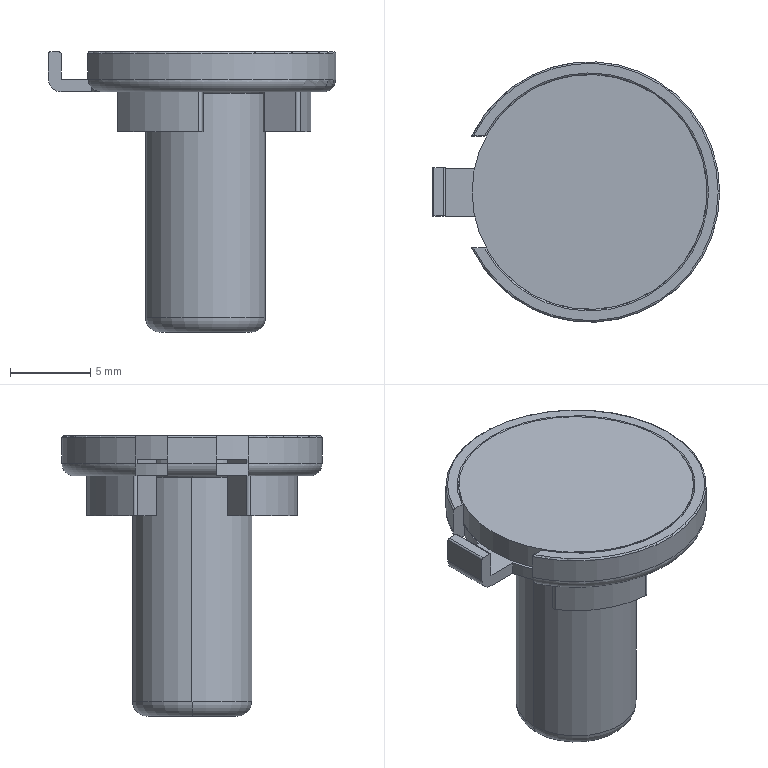NC program | NX | posted with a generic post | part box 17.958 x 16.273 x 17.5 mm
Lines 8183 to 8588 of 11029:
(刀补1 , TOOL : D4)
N16346 T04 M6
N16348 G54
N16350 G17 G0 G90 X3.736 Y7.769 S6500 M3
N16352 G43 Z30. H4
N16354 Z1.
N16356 G94 G1 X3.87 Y7.711 Z0.992 F1000.
N16358 X4.743 Y7.207 Z0.94
N16360 X5.551 Y6.604 Z0.887
N16362 X6.284 Y5.911 Z0.834
N16364 X6.931 Y5.138 Z0.781
N16366 X7.162 Y4.793 Z0.759
N16368 X7.279 Y4.617 Z0.748
N16370 X7.472 Y4.131 Z0.721
N16372 X7.546 Y3.613 Z0.693
N16374 X7.497 Y3.092 Z0.666
N16376 X7.328 Y2.597 Z0.638
N16378 X7.048 Y2.155 Z0.611
N16380 X6.673 Y1.791 Z0.584
N16382 X4.919 Y0.695 Z0.475
N16384 X4.963 Y0.382 Z0.459
N16386 Y-0.382 Z0.419
N16388 X4.919 Y-0.695 Z0.402
N16390 X6.673 Y-1.791 Z0.294
N16392 X7.048 Y-2.155 Z0.266
N16394 X7.328 Y-2.597 Z0.239
N16396 X7.497 Y-3.092 Z0.211
N16398 X7.546 Y-3.613 Z0.184
N16400 X7.472 Y-4.131 Z0.157
N16402 X7.279 Y-4.617 Z0.129
N16404 X7.162 Y-4.793 Z0.118
N16406 X6.931 Y-5.138 Z0.096
N16408 X6.284 Y-5.911 Z0.044
N16410 X5.551 Y-6.604 Z-0.009
N16412 X4.743 Y-7.207 Z-0.062
N16414 X3.87 Y-7.711 Z-0.115
N16416 X2.944 Y-8.11 Z-0.168
N16418 X1.977 Y-8.398 Z-0.221
N16420 X0.984 Y-8.571 Z-0.273
N16422 X0.359 Y-8.612 Z-0.306
N16424 X-0.158 Y-8.536 Z-0.334
N16426 X-0.644 Y-8.341 Z-0.361
N16428 X-1.07 Y-8.039 Z-0.389
N16430 X-1.415 Y-7.645 Z-0.416
N16432 X-1.657 Y-7.181 Z-0.443
N16434 X-1.786 Y-6.674 Z-0.471
N16436 X-1.858 Y-4.607 Z-0.579
N16438 X-2.15 Y-4.489 Z-0.596
N16440 X-2.812 Y-4.107 Z-0.636
N16442 X-3.061 Y-3.912 Z-0.652
N16444 X-4.887 Y-4.883 Z-0.761
N16446 X-5.39 Y-5.026 Z-0.788
N16448 X-5.913 Y-5.047 Z-0.816
N16450 X-6.426 Y-4.946 Z-0.843
N16452 X-6.902 Y-4.728 Z-0.87
N16454 X-7.313 Y-4.405 Z-0.898
N16456 X-7.638 Y-3.995 Z-0.925
N16458 X-7.731 Y-3.806 Z-0.936
N16460 X-7.915 Y-3.433 Z-0.958
N16462 X-8.261 Y-2.486 Z-1.011
N16464 X-8.495 Y-1.506 Z-1.064
N16466 X-8.613 Y-0.504 Z-1.117
N16468 Y0.504 Z-1.169
N16470 X-8.495 Y1.506 Z-1.222
N16472 X-8.261 Y2.486 Z-1.275
N16474 X-7.915 Y3.433 Z-1.328
N16476 X-7.731 Y3.806 Z-1.35
N16478 X-7.638 Y3.995 Z-1.361
N16480 X-7.313 Y4.405 Z-1.388
N16482 X-6.902 Y4.728 Z-1.416
N16484 X-6.426 Y4.946 Z-1.443
N16486 X-5.913 Y5.047 Z-1.47
N16488 X-5.39 Y5.026 Z-1.498
N16490 X-4.887 Y4.883 Z-1.525
N16492 X-3.061 Y3.912 Z-1.634
N16494 X-2.812 Y4.107 Z-1.65
N16496 X-2.15 Y4.489 Z-1.69
N16498 X-1.858 Y4.607 Z-1.707
N16500 X-1.829 Y5.431 Z-1.75
N16502 G41 X-1.808 Y5.529 D4
N16504 X-1.776 Y6.463
N16506 G2 X0.569 Y8.581 R2.2
N16508 X7.147 Y4.783 R8.6
N16510 X6.485 Y1.694 R2.2
N16512 G1 X4.9 Y0.703
N16514 G2 X4.9 Y-0.703 R4.95
N16516 G1 X6.485 Y-1.694
N16518 G2 X7.147 Y-4.783 R2.2
N16520 X0.569 Y-8.581 R8.6
N16522 X-1.776 Y-6.463 R2.2
N16524 G1 X-1.841 Y-4.595
N16526 G2 X-3.059 Y-3.892 R4.95
N16528 G1 X-4.709 Y-4.769
N16530 G2 X-7.716 Y-3.798 R2.2
N16532 X-7.716 Y3.798 R8.6
N16534 X-4.709 Y4.769 R2.2
N16536 G1 X-3.059 Y3.892
N16538 G2 X-1.841 Y4.595 R4.95
N16540 G1 X-1.808 Y5.529
N16542 X-1.779 Y6.375 Z-1.783
N16544 X-1.773 Y6.516 Z-1.788
N16546 X-1.76 Y6.656 Z-1.794
N16548 X-1.738 Y6.796 Z-1.799
N16550 X-1.708 Y6.933 Z-1.805
N16552 X-1.668 Y7.069 Z-1.81
N16554 X-1.62 Y7.202 Z-1.816
N16556 X-1.564 Y7.331 Z-1.821
N16558 X-1.499 Y7.456 Z-1.827
N16560 X-1.427 Y7.577 Z-1.832
N16562 X-1.347 Y7.693 Z-1.838
N16564 X-1.259 Y7.804 Z-1.843
N16566 X-1.165 Y7.909 Z-1.848
N16568 X-1.064 Y8.007 Z-1.854
N16570 X-0.957 Y8.1 Z-1.859
N16572 X-0.844 Y8.184 Z-1.865
N16574 X-0.726 Y8.262 Z-1.87
N16576 X-0.604 Y8.332 Z-1.876
N16578 X-0.477 Y8.393 Z-1.881
N16580 X-0.346 Y8.447 Z-1.887
N16582 X-0.213 Y8.492 Z-1.892
N16584 X-0.076 Y8.529 Z-1.898
N16586 X0.062 Y8.556 Z-1.903
N16588 X0.202 Y8.575 Z-1.909
N16590 X0.342 Y8.585 Z-1.914
N16592 X0.483 Z-1.92
N16594 X0.624 Y8.577 Z-1.925
N16596 X0.765 Y8.566 Z-1.93
N16598 X0.905 Y8.552 Z-1.936
N16600 X1.046 Y8.536 Z-1.941
N16602 X1.185 Y8.518 Z-1.947
N16604 X1.325 Y8.497 Z-1.952
N16606 X1.464 Y8.474 Z-1.958
N16608 X1.603 Y8.449 Z-1.963
N16610 X1.741 Y8.422 Z-1.969
N16612 X1.879 Y8.392 Z-1.974
N16614 X2.017 Y8.36 Z-1.98
N16616 X2.154 Y8.326 Z-1.985
N16618 X2.29 Y8.29 Z-1.991
N16620 X2.426 Y8.251 Z-1.996
N16622 X2.561 Y8.21 Z-2.002
N16624 X2.695 Y8.167 Z-2.007
N16626 X2.829 Y8.121 Z-2.013
N16628 X2.962 Y8.074 Z-2.018
N16630 X3.094 Y8.024 Z-2.023
N16632 X3.225 Y7.972 Z-2.029
N16634 X3.355 Y7.919 Z-2.034
N16636 X3.485 Y7.862 Z-2.04
N16638 X3.613 Y7.804 Z-2.045
N16640 X3.741 Y7.744 Z-2.051
N16642 X3.867 Y7.681 Z-2.056
N16644 X3.993 Y7.617 Z-2.062
N16646 X4.117 Y7.55 Z-2.067
N16648 X4.24 Y7.482 Z-2.073
N16650 X4.363 Y7.411 Z-2.078
N16652 X4.484 Y7.339 Z-2.084
N16654 X4.603 Y7.264 Z-2.089
N16656 X4.722 Y7.188 Z-2.095
N16658 X4.839 Y7.109 Z-2.1
N16660 X4.955 Y7.029 Z-2.105
N16662 X5.07 Y6.947 Z-2.111
N16664 X5.183 Y6.863 Z-2.116
N16666 X5.295 Y6.777 Z-2.122
N16668 X5.405 Y6.689 Z-2.127
N16670 X5.514 Y6.599 Z-2.133
N16672 X5.622 Y6.508 Z-2.138
N16674 X5.728 Y6.415 Z-2.144
N16676 X5.832 Y6.32 Z-2.149
N16678 X5.935 Y6.223 Z-2.155
N16680 X6.037 Y6.125 Z-2.16
N16682 X6.136 Y6.025 Z-2.166
N16684 X6.234 Y5.924 Z-2.171
N16686 X6.331 Y5.821 Z-2.177
N16688 X6.425 Y5.716 Z-2.182
N16690 X6.518 Y5.61 Z-2.188
N16692 X6.609 Y5.502 Z-2.193
N16694 X6.699 Y5.393 Z-2.198
N16696 X6.786 Y5.283 Z-2.204
N16698 X6.872 Y5.171 Z-2.209
N16700 X6.956 Y5.057 Z-2.215
N16702 X7.038 Y4.942 Z-2.22
N16704 X7.118 Y4.826 Z-2.226
N16706 X7.195 Y4.708 Z-2.231
N16708 X7.265 Y4.585 Z-2.237
N16710 X7.327 Y4.459 Z-2.242
N16712 X7.38 Y4.328 Z-2.248
N16714 X7.425 Y4.194 Z-2.253
N16716 X7.462 Y4.058 Z-2.259
N16718 X7.489 Y3.92 Z-2.264
N16720 X7.508 Y3.78 Z-2.27
N16722 X7.517 Y3.639 Z-2.275
N16724 X7.518 Y3.498 Z-2.28
N16726 X7.51 Y3.357 Z-2.286
N16728 X7.492 Y3.217 Z-2.291
N16730 X7.466 Y3.079 Z-2.297
N16732 X7.431 Y2.942 Z-2.302
N16734 X7.387 Y2.808 Z-2.308
N16736 X7.334 Y2.677 Z-2.313
N16738 X7.274 Y2.55 Z-2.319
N16740 X7.205 Y2.427 Z-2.324
N16742 X7.128 Y2.308 Z-2.33
N16744 X7.044 Y2.195 Z-2.335
N16746 X6.953 Y2.087 Z-2.341
N16748 X6.856 Y1.985 Z-2.346
N16750 X6.752 Y1.89 Z-2.352
N16752 X6.642 Y1.801 Z-2.357
N16754 X6.526 Y1.72 Z-2.363
N16756 X6.407 Y1.645 Z-2.368
N16758 X6.287 Y1.57 Z-2.373
N16760 X5.091 Y0.823 Z-2.428
N16762 X4.902 Y0.704 Z-2.437
N16764 X4.908 Y0.647 Z-2.439
N16766 X4.924 Y0.507 Z-2.445
N16768 X4.936 Y0.366 Z-2.45
N16770 X4.945 Y0.225 Z-2.455
N16772 X4.949 Y0.084 Z-2.461
N16774 X4.95 Y-0.057 Z-2.466
N16776 X4.946 Y-0.198 Z-2.472
N16778 X4.938 Y-0.339 Z-2.477
N16780 X4.927 Y-0.479 Z-2.483
N16782 X4.907 Y-0.708 Z-2.492
N16784 X4.948 Y-0.733 Z-2.494
N16786 X5.067 Y-0.808 Z-2.499
N16788 X5.187 Y-0.882 Z-2.505
N16790 X5.307 Y-0.958 Z-2.51
N16792 X5.426 Y-1.032 Z-2.516
N16794 X5.546 Y-1.107 Z-2.521
N16796 X6.383 Y-1.63 Z-2.559
N16798 X6.503 Y-1.705 Z-2.565
N16800 X6.62 Y-1.785 Z-2.57
N16802 X6.731 Y-1.872 Z-2.576
N16804 X6.836 Y-1.966 Z-2.581
N16806 X6.935 Y-2.066 Z-2.587
N16808 X7.027 Y-2.173 Z-2.592
N16810 X7.112 Y-2.285 Z-2.598
N16812 X7.191 Y-2.403 Z-2.603
N16814 X7.261 Y-2.525 Z-2.609
N16816 X7.323 Y-2.652 Z-2.614
N16818 X7.377 Y-2.782 Z-2.62
N16820 X7.423 Y-2.916 Z-2.625
N16822 X7.46 Y-3.052 Z-2.63
N16824 X7.488 Y-3.19 Z-2.636
N16826 X7.507 Y-3.33 Z-2.641
N16828 X7.517 Y-3.47 Z-2.647
N16830 X7.518 Y-3.612 Z-2.652
N16832 X7.51 Y-3.752 Z-2.658
N16834 X7.494 Y-3.892 Z-2.663
N16836 X7.468 Y-4.031 Z-2.669
N16838 X7.433 Y-4.168 Z-2.674
N16840 X7.39 Y-4.302 Z-2.68
N16842 X7.338 Y-4.433 Z-2.685
N16844 X7.278 Y-4.561 Z-2.691
N16846 X7.21 Y-4.684 Z-2.696
N16848 X7.134 Y-4.803 Z-2.702
N16850 X7.054 Y-4.92 Z-2.707
N16852 X6.972 Y-5.035 Z-2.713
N16854 X6.889 Y-5.148 Z-2.718
N16856 X6.803 Y-5.261 Z-2.723
N16858 X6.716 Y-5.372 Z-2.729
N16860 X6.627 Y-5.481 Z-2.734
N16862 X6.536 Y-5.589 Z-2.74
N16864 X6.444 Y-5.696 Z-2.745
N16866 X6.349 Y-5.8 Z-2.751
N16868 X6.253 Y-5.904 Z-2.756
N16870 X6.156 Y-6.006 Z-2.762
N16872 X6.056 Y-6.106 Z-2.767
N16874 X5.955 Y-6.204 Z-2.773
N16876 X5.853 Y-6.301 Z-2.778
N16878 X5.749 Y-6.396 Z-2.784
N16880 X5.643 Y-6.49 Z-2.789
N16882 X5.536 Y-6.582 Z-2.795
N16884 X5.427 Y-6.671 Z-2.8
N16886 X5.317 Y-6.76 Z-2.805
N16888 X5.205 Y-6.846 Z-2.811
N16890 X5.092 Y-6.93 Z-2.816
N16892 X4.978 Y-7.013 Z-2.822
N16894 X4.862 Y-7.094 Z-2.827
N16896 X4.745 Y-7.173 Z-2.833
N16898 X4.627 Y-7.249 Z-2.838
N16900 X4.507 Y-7.324 Z-2.844
N16902 X4.386 Y-7.397 Z-2.849
N16904 X4.264 Y-7.468 Z-2.855
N16906 X4.141 Y-7.537 Z-2.86
N16908 X4.017 Y-7.604 Z-2.866
N16910 X3.892 Y-7.669 Z-2.871
N16912 X3.766 Y-7.732 Z-2.877
N16914 X3.638 Y-7.793 Z-2.882
N16916 X3.51 Y-7.851 Z-2.888
N16918 X3.381 Y-7.908 Z-2.893
N16920 X3.25 Y-7.962 Z-2.898
N16922 X3.119 Y-8.014 Z-2.904
N16924 X2.987 Y-8.064 Z-2.909
N16926 X2.855 Y-8.112 Z-2.915
N16928 X2.721 Y-8.158 Z-2.92
N16930 X2.587 Y-8.202 Z-2.926
N16932 X2.452 Y-8.243 Z-2.931
N16934 X2.317 Y-8.282 Z-2.937
N16936 X2.18 Y-8.319 Z-2.942
N16938 X2.044 Y-8.354 Z-2.948
N16940 X1.906 Y-8.386 Z-2.953
N16942 X1.769 Y-8.416 Z-2.959
N16944 X1.63 Y-8.444 Z-2.964
N16946 X1.491 Y-8.47 Z-2.97
N16948 X1.352 Y-8.493 Z-2.975
N16950 X1.213 Y-8.514 Z-2.98
N16952 X1.073 Y-8.533 Z-2.986
N16954 X0.933 Y-8.549 Z-2.991
N16956 X0.792 Y-8.563 Z-2.997
N16958 X0.652 Y-8.575 Z-3.002
N16960 X0.511 Y-8.584 Z-3.008
N16962 X0.37 Y-8.585 Z-3.013
N16964 X0.229 Y-8.577 Z-3.019
N16966 X0.089 Y-8.561 Z-3.024
N16968 X-0.05 Y-8.535 Z-3.03
N16970 X-0.186 Y-8.5 Z-3.035
N16972 X-0.321 Y-8.457 Z-3.041
N16974 X-0.452 Y-8.405 Z-3.046
N16976 X-0.579 Y-8.344 Z-3.052
N16978 X-0.703 Y-8.276 Z-3.057
N16980 X-0.822 Y-8.2 Z-3.063
N16982 X-0.935 Y-8.117 Z-3.068
N16984 X-1.044 Y-8.026 Z-3.073
N16986 X-1.145 Y-7.929 Z-3.079
N16988 X-1.241 Y-7.825 Z-3.084
N16990 X-1.33 Y-7.715 Z-3.09
N16992 X-1.411 Y-7.6 Z-3.095
N16994 X-1.486 Y-7.48 Z-3.101
N16996 X-1.552 Y-7.356 Z-3.106
N16998 X-1.61 Y-7.227 Z-3.112
N17000 X-1.66 Y-7.095 Z-3.117
N17002 X-1.701 Y-6.96 Z-3.123
N17004 X-1.733 Y-6.823 Z-3.128
N17006 X-1.757 Y-6.684 Z-3.134
N17008 X-1.771 Y-6.543 Z-3.139
N17010 X-1.778 Y-6.403 Z-3.145
N17012 X-1.783 Y-6.262 Z-3.15
N17014 X-1.832 Y-4.851 Z-3.205
N17016 X-1.841 Y-4.596 Z-3.215
N17018 X-1.994 Y-4.53 Z-3.221
N17020 X-2.123 Y-4.472 Z-3.227
N17022 X-2.249 Y-4.409 Z-3.232
N17024 X-2.374 Y-4.344 Z-3.238
N17026 X-2.497 Y-4.274 Z-3.243
N17028 X-2.618 Y-4.201 Z-3.248
N17030 X-2.736 Y-4.125 Z-3.254
N17032 X-2.853 Y-4.045 Z-3.259
N17034 X-3.069 Y-3.897 Z-3.27
N17036 X-3.206 Y-3.97 Z-3.276
N17038 X-4.327 Y-4.566 Z-3.325
N17040 X-4.451 Y-4.633 Z-3.33
N17042 X-4.576 Y-4.698 Z-3.336
N17044 X-4.701 Y-4.765 Z-3.341
N17046 X-4.827 Y-4.827 Z-3.347
N17048 X-4.957 Y-4.882 Z-3.352
N17050 X-5.09 Y-4.928 Z-3.358
N17052 X-5.226 Y-4.965 Z-3.363
N17054 X-5.365 Y-4.994 Z-3.369
N17056 X-5.504 Y-5.014 Z-3.374
N17058 X-5.645 Y-5.024 Z-3.38
N17060 X-5.786 Y-5.026 Z-3.385
N17062 X-5.927 Y-5.019 Z-3.391
N17064 X-6.067 Y-5.002 Z-3.396
N17066 X-6.206 Y-4.977 Z-3.402
N17068 X-6.343 Y-4.943 Z-3.407
N17070 X-6.477 Y-4.9 Z-3.413
N17072 X-6.608 Y-4.849 Z-3.418
N17074 X-6.736 Y-4.789 Z-3.423
N17076 X-6.86 Y-4.721 Z-3.429
N17078 X-6.979 Y-4.646 Z-3.434
N17080 X-7.093 Y-4.563 Z-3.44
N17082 X-7.202 Y-4.473 Z-3.445
N17084 X-7.304 Y-4.376 Z-3.451
N17086 X-7.4 Y-4.272 Z-3.456
N17088 X-7.489 Y-4.163 Z-3.462
N17090 X-7.571 Y-4.048 Z-3.467
N17092 X-7.646 Y-3.929 Z-3.473
N17094 X-7.713 Y-3.804 Z-3.478
N17096 X-7.774 Y-3.677 Z-3.484
N17098 X-7.833 Y-3.549 Z-3.489
N17100 X-7.891 Y-3.42 Z-3.495
N17102 X-7.946 Y-3.29 Z-3.5
N17104 G2 X-7.716 Y3.798 R8.6
N17106 X-4.709 Y4.769 R2.2
N17108 G1 X-3.059 Y3.892
N17110 G2 X-1.841 Y4.595 R4.95
N17112 G1 X-1.776 Y6.463
N17114 G2 X0.569 Y8.581 R2.2
N17116 X7.147 Y4.783 R8.6
N17118 X6.485 Y1.694 R2.2
N17120 G1 X4.9 Y0.703
N17122 G2 X4.9 Y-0.703 R4.95
N17124 G1 X6.485 Y-1.694
N17126 G2 X7.147 Y-4.783 R2.2
N17128 X0.569 Y-8.581 R8.6
N17130 X-1.776 Y-6.463 R2.2
N17132 G1 X-1.841 Y-4.595
N17134 G2 X-3.059 Y-3.892 R4.95
N17136 G1 X-4.709 Y-4.769
N17138 G2 X-7.716 Y-3.798 R2.2
N17140 X-7.946 Y-3.29 R8.6
N17142 G40
N17144 G1 X-7.999 Y-3.206
N17146 Z-2.5
N17148 G0 Z30.
N17150 M5